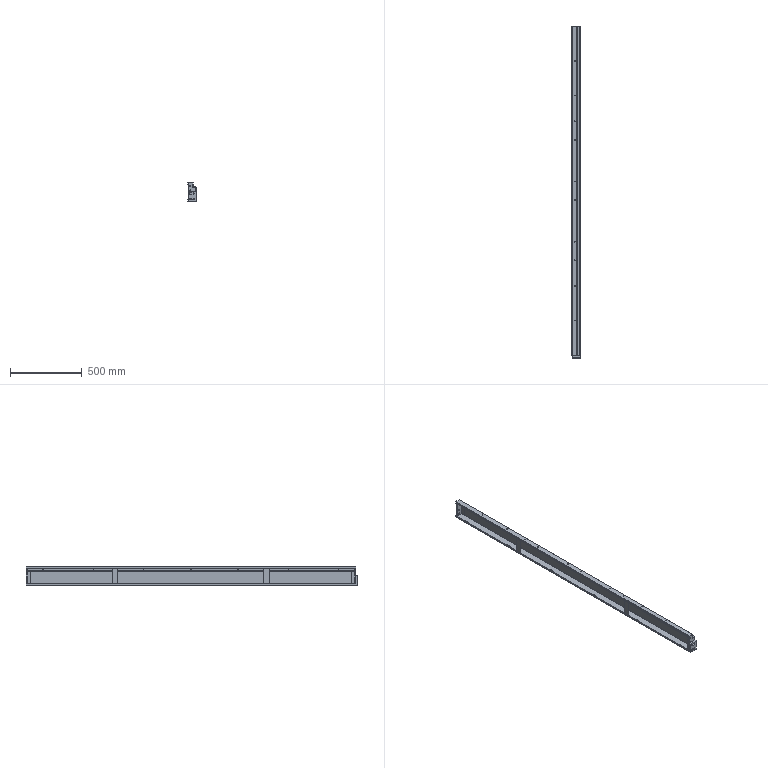Part | 6 solids | 238 faces | box 58 x 2316 x 130 mm | volume 819445 mm3 | plane 132 | cylinder 106 | commonest cylinder face diameters 5 x32 8 x20 9 x18 4.6 x14 2 x10 4.4 x6